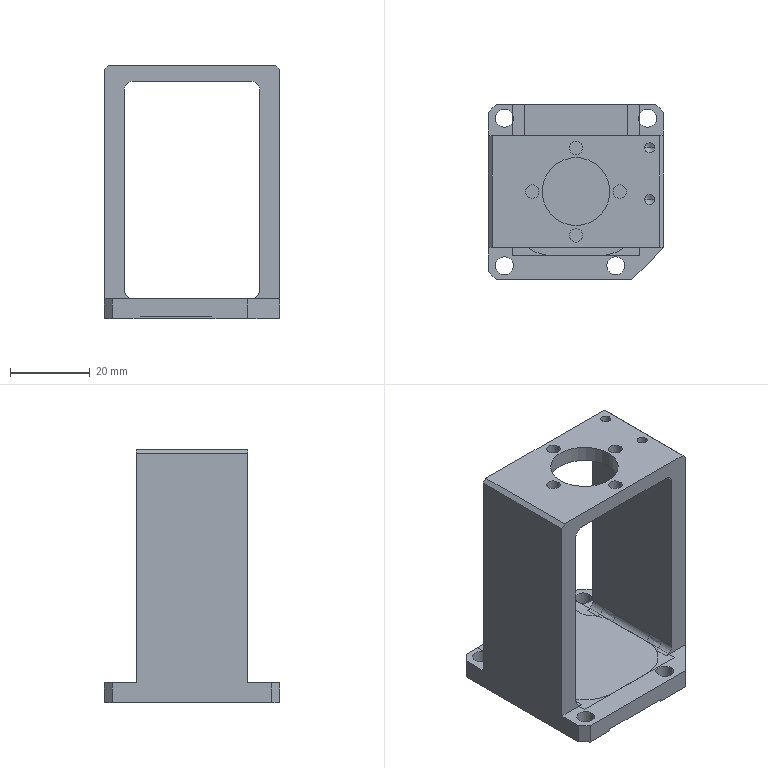NC program | NX | posted with a generic post | part box 44 x 44 x 63.6 mm
Lines 1 to 61 of 4011:
N10 G17 G21 G94 G90
(FLOOR_WALL , TOOL : D63)
N12 T01 M6
N14 G54
N16 G17 G0 G90 X58.5 Y0. B0. C0. S6500 M3
N18 G43 Z30. H1
N20 Z3.
N22 G94 G1 Z0. F1500.
N24 X55.5
N26 X-55.5
N28 X-58.5
N30 Z3.
N32 G0 Z30.
N34 M5
(DRILLING , TOOL : D6A45)
N36 T07 M6
N38 G54
N40 G17 G0 G90 X0. Y11. B0. C0. S5000 M3
N42 G43 Z30. H7
N44 G94 G81 G98 Z-1.6 F250. R3.
N46 X11. Y0.
N48 X0. Y-11.
N50 Y0.
N52 X-11.
N54 X-18.5 Y2.
N56 Y-11.
N58 G80
N60 G0 X-18.5 Y-11. Z30.
N62 M5
(DRILLING_COPY , TOOL : 2.5ZT)
N64 T09 M6
N66 G54
N68 G17 G0 G90 X-18.5 Y-11. B0. C0. S2000 M3
N70 G43 Z30. H9
N72 G94 G83 G98 Z-8.251 F80. Q2. R3.
N74 Y2.
N76 G80
N78 G0 X-18.5 Y2. Z30.
N80 M5
(DRILLING_COPY_COPY , TOOL : 3.4ZT)
N82 T08 M6
N84 G54
N86 G17 G0 G90 X11. Y0. B0. C0. S2000 M3
N88 G43 Z30. H8
N90 G94 G83 G98 Z-6.521 F150. Q2. R3.
N92 X0. Y-11.
N94 X-11. Y0.
N96 X0. Y11.
N98 G80
N100 G0 X0. Y11. Z30.
N102 M5